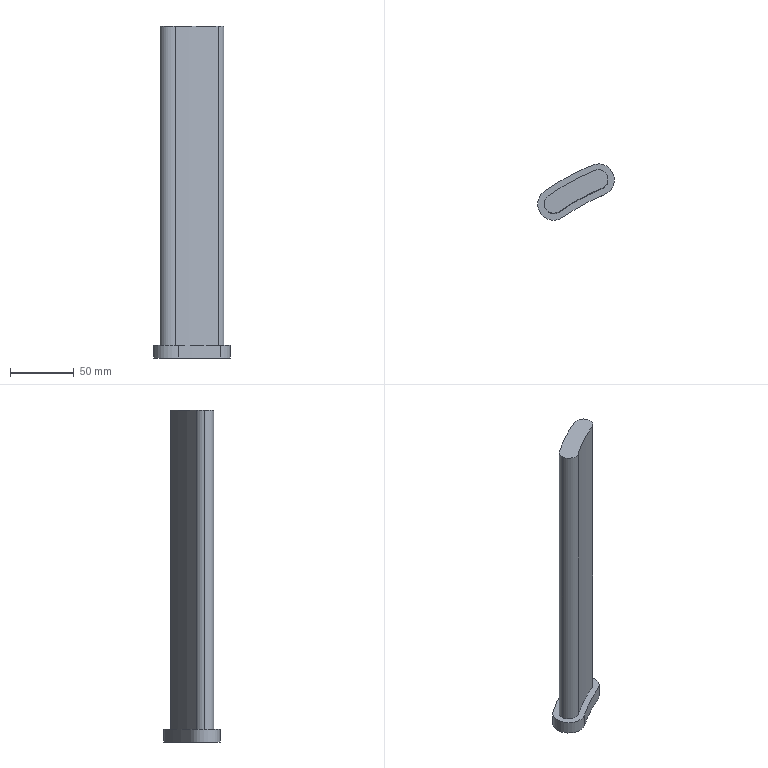Part | SolidWorks | features Extrusion 1, ICE 1 | 1 solid | 13 faces | box 60.075 x 44.074 x 260 mm | volume 209087 mm3 | cylinder 10 | plane 3 | commonest cylinder face diameters 15 x3 25 x3 355 x1 365 x1 395 x1 405 x1
STEP:
#1=CARTESIAN_POINT('',(-351.814,358.26,-240.));
#2=VERTEX_POINT('',#1);
#3=CARTESIAN_POINT('',(-359.529,346.712,-240.));
#4=VERTEX_POINT('',#3);
#5=CARTESIAN_POINT('',(-364.314,358.26,-240.));
#6=DIRECTION('',(0.,0.,-1.));
#7=DIRECTION('',(-1.,0.,0.));
#8=AXIS2_PLACEMENT_3D('',#5,#6,#7);
#9=CIRCLE('',#8,12.5);
#10=EDGE_CURVE('',#2,#4,#9,.T.);
#11=ORIENTED_EDGE('',*,*,#10,.F.);
#12=CARTESIAN_POINT('',(-351.814,358.26,-230.));
#13=VERTEX_POINT('',#12);
#14=CARTESIAN_POINT('',(-351.814,358.26,-240.));
#15=DIRECTION('',(0.,0.,1.));
#16=VECTOR('',#15,1000.);
#17=LINE('',#14,#16);
#18=EDGE_CURVE('',#2,#13,#17,.T.);
#19=ORIENTED_EDGE('',*,*,#18,.T.);
#20=CARTESIAN_POINT('',(-359.529,346.712,-230.));
#21=VERTEX_POINT('',#20);
#22=CARTESIAN_POINT('',(-364.314,358.26,-230.));
#23=DIRECTION('',(0.,0.,-1.));
#24=DIRECTION('',(-1.,0.,0.));
#25=AXIS2_PLACEMENT_3D('',#22,#23,#24);
#26=CIRCLE('',#25,12.5);
#27=EDGE_CURVE('',#13,#21,#26,.T.);
#28=ORIENTED_EDGE('',*,*,#27,.T.);
#29=CARTESIAN_POINT('',(-359.529,346.712,-240.));
#30=DIRECTION('',(0.,0.,1.));
#31=VECTOR('',#30,1000.);
#32=LINE('',#29,#31);
#33=EDGE_CURVE('',#4,#21,#32,.T.);
#34=ORIENTED_EDGE('',*,*,#33,.F.);
#35=EDGE_LOOP('',(#11,#19,#28,#34));
#36=FACE_OUTER_BOUND('',#35,.T.);
#37=CARTESIAN_POINT('',(-364.314,358.26,-240.));
#38=DIRECTION('',(0.,0.,1.));
#39=DIRECTION('',(1.,0.,0.));
#40=AXIS2_PLACEMENT_3D('',#37,#38,#39);
#41=CYLINDRICAL_SURFACE('',#40,12.5);
#42=ADVANCED_FACE('',(#36),#41,.T.);
#43=CARTESIAN_POINT('',(-406.89,339.186,20.));
#44=VERTEX_POINT('',#43);
#45=CARTESIAN_POINT('',(-395.134,333.01,20.));
#46=VERTEX_POINT('',#45);
#47=CARTESIAN_POINT('',(-399.39,339.186,20.));
#48=DIRECTION('',(0.,0.,1.));
#49=DIRECTION('',(1.,0.,0.));
#50=AXIS2_PLACEMENT_3D('',#47,#48,#49);
#51=CIRCLE('',#50,7.5);
#52=EDGE_CURVE('',#44,#46,#51,.T.);
#53=ORIENTED_EDGE('',*,*,#52,.F.);
#54=CARTESIAN_POINT('',(-406.89,339.186,-230.));
#55=VERTEX_POINT('',#54);
#56=CARTESIAN_POINT('',(-406.89,339.186,20.));
#57=DIRECTION('',(0.,0.,-1.));
#58=VECTOR('',#57,1000.);
#59=LINE('',#56,#58);
#60=EDGE_CURVE('',#44,#55,#59,.T.);
#61=ORIENTED_EDGE('',*,*,#60,.T.);
#62=CARTESIAN_POINT('',(-395.134,333.01,-230.));
#63=VERTEX_POINT('',#62);
#64=CARTESIAN_POINT('',(-399.39,339.186,-230.));
#65=DIRECTION('',(0.,0.,-1.));
#66=DIRECTION('',(1.,0.,0.));
#67=AXIS2_PLACEMENT_3D('',#64,#65,#66);
#68=CIRCLE('',#67,7.5);
#69=EDGE_CURVE('',#63,#55,#68,.T.);
#70=ORIENTED_EDGE('',*,*,#69,.F.);
#71=CARTESIAN_POINT('',(-395.134,333.01,20.));
#72=DIRECTION('',(0.,0.,-1.));
#73=VECTOR('',#72,1000.);
#74=LINE('',#71,#73);
#75=EDGE_CURVE('',#46,#63,#74,.T.);
#76=ORIENTED_EDGE('',*,*,#75,.F.);
#77=EDGE_LOOP('',(#53,#61,#70,#76));
#78=FACE_OUTER_BOUND('',#77,.T.);
#79=CARTESIAN_POINT('',(-399.39,339.186,20.));
#80=DIRECTION('',(0.,0.,-1.));
#81=DIRECTION('',(-1.,0.,0.));
#82=AXIS2_PLACEMENT_3D('',#79,#80,#81);
#83=CYLINDRICAL_SURFACE('',#82,7.5);
#84=ADVANCED_FACE('',(#78),#83,.T.);
#85=CARTESIAN_POINT('',(-361.443,351.331,20.));
#86=VERTEX_POINT('',#85);
#87=CARTESIAN_POINT('',(-361.443,351.331,-230.));
#88=VERTEX_POINT('',#87);
#89=CARTESIAN_POINT('',(-361.443,351.331,20.));
#90=DIRECTION('',(0.,0.,-1.));
#91=VECTOR('',#90,1000.);
#92=LINE('',#89,#91);
#93=EDGE_CURVE('',#86,#88,#92,.T.);
#94=ORIENTED_EDGE('',*,*,#93,.T.);
#95=CARTESIAN_POINT('',(-367.185,365.189,-230.));
#96=VERTEX_POINT('',#95);
#97=CARTESIAN_POINT('',(-364.314,358.26,-230.));
#98=DIRECTION('',(0.,0.,-1.));
#99=DIRECTION('',(1.,0.,0.));
#100=AXIS2_PLACEMENT_3D('',#97,#98,#99);
#101=CIRCLE('',#100,7.5);
#102=EDGE_CURVE('',#96,#88,#101,.T.);
#103=ORIENTED_EDGE('',*,*,#102,.F.);
#104=CARTESIAN_POINT('',(-367.185,365.189,20.));
#105=VERTEX_POINT('',#104);
#106=CARTESIAN_POINT('',(-367.185,365.189,20.));
#107=DIRECTION('',(0.,0.,-1.));
#108=VECTOR('',#107,1000.);
#109=LINE('',#106,#108);
#110=EDGE_CURVE('',#105,#96,#109,.T.);
#111=ORIENTED_EDGE('',*,*,#110,.F.);
#112=CARTESIAN_POINT('',(-364.314,358.26,20.));
#113=DIRECTION('',(0.,0.,1.));
#114=DIRECTION('',(1.,0.,0.));
#115=AXIS2_PLACEMENT_3D('',#112,#113,#114);
#116=CIRCLE('',#115,7.5);
#117=EDGE_CURVE('',#86,#105,#116,.T.);
#118=ORIENTED_EDGE('',*,*,#117,.F.);
#119=EDGE_LOOP('',(#94,#103,#111,#118));
#120=FACE_OUTER_BOUND('',#119,.T.);
#121=CARTESIAN_POINT('',(-364.314,358.26,20.));
#122=DIRECTION('',(0.,0.,-1.));
#123=DIRECTION('',(-1.,0.,0.));
#124=AXIS2_PLACEMENT_3D('',#121,#122,#123);
#125=CYLINDRICAL_SURFACE('',#124,7.5);
#126=ADVANCED_FACE('',(#120),#125,.T.);
#127=ORIENTED_EDGE('',*,*,#110,.T.);
#128=CARTESIAN_POINT('',(-403.645,345.362,-230.));
#129=VERTEX_POINT('',#128);
#130=CARTESIAN_POINT('',(-291.585,182.731,-230.));
#131=DIRECTION('',(0.,0.,-1.));
#132=DIRECTION('',(1.,0.,0.));
#133=AXIS2_PLACEMENT_3D('',#130,#131,#132);
#134=CIRCLE('',#133,197.5);
#135=EDGE_CURVE('',#129,#96,#134,.T.);
#136=ORIENTED_EDGE('',*,*,#135,.F.);
#137=CARTESIAN_POINT('',(-403.645,345.362,20.));
#138=VERTEX_POINT('',#137);
#139=CARTESIAN_POINT('',(-403.645,345.362,20.));
#140=DIRECTION('',(0.,0.,-1.));
#141=VECTOR('',#140,1000.);
#142=LINE('',#139,#141);
#143=EDGE_CURVE('',#138,#129,#142,.T.);
#144=ORIENTED_EDGE('',*,*,#143,.F.);
#145=CARTESIAN_POINT('',(-291.585,182.731,20.));
#146=DIRECTION('',(0.,0.,1.));
#147=DIRECTION('',(1.,0.,0.));
#148=AXIS2_PLACEMENT_3D('',#145,#146,#147);
#149=CIRCLE('',#148,197.5);
#150=EDGE_CURVE('',#105,#138,#149,.T.);
#151=ORIENTED_EDGE('',*,*,#150,.F.);
#152=EDGE_LOOP('',(#127,#136,#144,#151));
#153=FACE_OUTER_BOUND('',#152,.T.);
#154=CARTESIAN_POINT('',(-291.585,182.731,20.));
#155=DIRECTION('',(0.,0.,-1.));
#156=DIRECTION('',(-1.,0.,0.));
#157=AXIS2_PLACEMENT_3D('',#154,#155,#156);
#158=CYLINDRICAL_SURFACE('',#157,197.5);
#159=ADVANCED_FACE('',(#153),#158,.T.);
#160=ORIENTED_EDGE('',*,*,#60,.F.);
#161=CARTESIAN_POINT('',(-399.39,339.186,20.));
#162=DIRECTION('',(0.,0.,1.));
#163=DIRECTION('',(1.,0.,0.));
#164=AXIS2_PLACEMENT_3D('',#161,#162,#163);
#165=CIRCLE('',#164,7.5);
#166=EDGE_CURVE('',#138,#44,#165,.T.);
#167=ORIENTED_EDGE('',*,*,#166,.F.);
#168=ORIENTED_EDGE('',*,*,#143,.T.);
#169=CARTESIAN_POINT('',(-399.39,339.186,-230.));
#170=DIRECTION('',(0.,0.,-1.));
#171=DIRECTION('',(1.,0.,0.));
#172=AXIS2_PLACEMENT_3D('',#169,#170,#171);
#173=CIRCLE('',#172,7.5);
#174=EDGE_CURVE('',#55,#129,#173,.T.);
#175=ORIENTED_EDGE('',*,*,#174,.F.);
#176=EDGE_LOOP('',(#160,#167,#168,#175));
#177=FACE_OUTER_BOUND('',#176,.T.);
#178=CARTESIAN_POINT('',(-399.39,339.186,20.));
#179=DIRECTION('',(0.,0.,-1.));
#180=DIRECTION('',(-1.,0.,0.));
#181=AXIS2_PLACEMENT_3D('',#178,#179,#180);
#182=CYLINDRICAL_SURFACE('',#181,7.5);
#183=ADVANCED_FACE('',(#177),#182,.T.);
#184=ORIENTED_EDGE('',*,*,#75,.T.);
#185=CARTESIAN_POINT('',(-291.585,182.731,-230.));
#186=DIRECTION('',(0.,0.,1.));
#187=DIRECTION('',(1.,0.,0.));
#188=AXIS2_PLACEMENT_3D('',#185,#186,#187);
#189=CIRCLE('',#188,182.5);
#190=EDGE_CURVE('',#88,#63,#189,.T.);
#191=ORIENTED_EDGE('',*,*,#190,.F.);
#192=ORIENTED_EDGE('',*,*,#93,.F.);
#193=CARTESIAN_POINT('',(-291.585,182.731,20.));
#194=DIRECTION('',(0.,0.,-1.));
#195=DIRECTION('',(1.,0.,0.));
#196=AXIS2_PLACEMENT_3D('',#193,#194,#195);
#197=CIRCLE('',#196,182.5);
#198=EDGE_CURVE('',#46,#86,#197,.T.);
#199=ORIENTED_EDGE('',*,*,#198,.F.);
#200=EDGE_LOOP('',(#184,#191,#192,#199));
#201=FACE_OUTER_BOUND('',#200,.T.);
#202=CARTESIAN_POINT('',(-291.585,182.731,20.));
#203=DIRECTION('',(0.,0.,-1.));
#204=DIRECTION('',(-1.,0.,0.));
#205=AXIS2_PLACEMENT_3D('',#202,#203,#204);
#206=CYLINDRICAL_SURFACE('',#205,182.5);
#207=ADVANCED_FACE('',(#201),#206,.F.);
#208=ORIENTED_EDGE('',*,*,#117,.T.);
#209=ORIENTED_EDGE('',*,*,#150,.T.);
#210=ORIENTED_EDGE('',*,*,#166,.T.);
#211=ORIENTED_EDGE('',*,*,#52,.T.);
#212=ORIENTED_EDGE('',*,*,#198,.T.);
#213=EDGE_LOOP('',(#208,#209,#210,#211,#212));
#214=FACE_OUTER_BOUND('',#213,.T.);
#215=CARTESIAN_POINT('',(-327.95,270.495,20.));
#216=DIRECTION('',(0.,0.,1.));
#217=DIRECTION('',(1.,0.,0.));
#218=AXIS2_PLACEMENT_3D('',#215,#216,#217);
#219=PLANE('',#218);
#220=ADVANCED_FACE('',(#214),#219,.T.);
#221=CARTESIAN_POINT('',(-392.297,328.893,-230.));
#222=VERTEX_POINT('',#221);
#223=CARTESIAN_POINT('',(-406.482,349.479,-230.));
#224=VERTEX_POINT('',#223);
#225=CARTESIAN_POINT('',(-399.39,339.186,-230.));
#226=DIRECTION('',(0.,0.,-1.));
#227=DIRECTION('',(-1.,0.,0.));
#228=AXIS2_PLACEMENT_3D('',#225,#226,#227);
#229=CIRCLE('',#228,12.5);
#230=EDGE_CURVE('',#222,#224,#229,.T.);
#231=ORIENTED_EDGE('',*,*,#230,.T.);
#232=CARTESIAN_POINT('',(-406.482,349.479,-240.));
#233=VERTEX_POINT('',#232);
#234=CARTESIAN_POINT('',(-406.482,349.479,-240.));
#235=DIRECTION('',(0.,0.,1.));
#236=VECTOR('',#235,1000.);
#237=LINE('',#234,#236);
#238=EDGE_CURVE('',#233,#224,#237,.T.);
#239=ORIENTED_EDGE('',*,*,#238,.F.);
#240=CARTESIAN_POINT('',(-392.297,328.893,-240.));
#241=VERTEX_POINT('',#240);
#242=CARTESIAN_POINT('',(-399.39,339.186,-240.));
#243=DIRECTION('',(0.,0.,-1.));
#244=DIRECTION('',(-1.,0.,0.));
#245=AXIS2_PLACEMENT_3D('',#242,#243,#244);
#246=CIRCLE('',#245,12.5);
#247=EDGE_CURVE('',#241,#233,#246,.T.);
#248=ORIENTED_EDGE('',*,*,#247,.F.);
#249=CARTESIAN_POINT('',(-392.297,328.893,-240.));
#250=DIRECTION('',(0.,0.,1.));
#251=VECTOR('',#250,1000.);
#252=LINE('',#249,#251);
#253=EDGE_CURVE('',#241,#222,#252,.T.);
#254=ORIENTED_EDGE('',*,*,#253,.T.);
#255=EDGE_LOOP('',(#231,#239,#248,#254));
#256=FACE_OUTER_BOUND('',#255,.T.);
#257=CARTESIAN_POINT('',(-399.39,339.186,-240.));
#258=DIRECTION('',(0.,0.,1.));
#259=DIRECTION('',(1.,0.,0.));
#260=AXIS2_PLACEMENT_3D('',#257,#258,#259);
#261=CYLINDRICAL_SURFACE('',#260,12.5);
#262=ADVANCED_FACE('',(#256),#261,.T.);
#263=CARTESIAN_POINT('',(-369.099,369.808,-230.));
#264=VERTEX_POINT('',#263);
#265=CARTESIAN_POINT('',(-291.585,182.731,-230.));
#266=DIRECTION('',(0.,0.,-1.));
#267=DIRECTION('',(-1.,0.,0.));
#268=AXIS2_PLACEMENT_3D('',#265,#266,#267);
#269=CIRCLE('',#268,202.5);
#270=EDGE_CURVE('',#224,#264,#269,.T.);
#271=ORIENTED_EDGE('',*,*,#270,.T.);
#272=CARTESIAN_POINT('',(-369.099,369.808,-240.));
#273=VERTEX_POINT('',#272);
#274=CARTESIAN_POINT('',(-369.099,369.808,-240.));
#275=DIRECTION('',(0.,0.,1.));
#276=VECTOR('',#275,1000.);
#277=LINE('',#274,#276);
#278=EDGE_CURVE('',#273,#264,#277,.T.);
#279=ORIENTED_EDGE('',*,*,#278,.F.);
#280=CARTESIAN_POINT('',(-291.585,182.731,-240.));
#281=DIRECTION('',(0.,0.,-1.));
#282=DIRECTION('',(-1.,0.,0.));
#283=AXIS2_PLACEMENT_3D('',#280,#281,#282);
#284=CIRCLE('',#283,202.5);
#285=EDGE_CURVE('',#233,#273,#284,.T.);
#286=ORIENTED_EDGE('',*,*,#285,.F.);
#287=ORIENTED_EDGE('',*,*,#238,.T.);
#288=EDGE_LOOP('',(#271,#279,#286,#287));
#289=FACE_OUTER_BOUND('',#288,.T.);
#290=CARTESIAN_POINT('',(-291.585,182.731,-240.));
#291=DIRECTION('',(0.,0.,1.));
#292=DIRECTION('',(1.,0.,0.));
#293=AXIS2_PLACEMENT_3D('',#290,#291,#292);
#294=CYLINDRICAL_SURFACE('',#293,202.5);
#295=ADVANCED_FACE('',(#289),#294,.T.);
#296=ORIENTED_EDGE('',*,*,#18,.F.);
#297=CARTESIAN_POINT('',(-364.314,358.26,-240.));
#298=DIRECTION('',(0.,0.,-1.));
#299=DIRECTION('',(-1.,0.,0.));
#300=AXIS2_PLACEMENT_3D('',#297,#298,#299);
#301=CIRCLE('',#300,12.5);
#302=EDGE_CURVE('',#273,#2,#301,.T.);
#303=ORIENTED_EDGE('',*,*,#302,.F.);
#304=ORIENTED_EDGE('',*,*,#278,.T.);
#305=CARTESIAN_POINT('',(-364.314,358.26,-230.));
#306=DIRECTION('',(0.,0.,-1.));
#307=DIRECTION('',(-1.,0.,0.));
#308=AXIS2_PLACEMENT_3D('',#305,#306,#307);
#309=CIRCLE('',#308,12.5);
#310=EDGE_CURVE('',#264,#13,#309,.T.);
#311=ORIENTED_EDGE('',*,*,#310,.T.);
#312=EDGE_LOOP('',(#296,#303,#304,#311));
#313=FACE_OUTER_BOUND('',#312,.T.);
#314=CARTESIAN_POINT('',(-364.314,358.26,-240.));
#315=DIRECTION('',(0.,0.,1.));
#316=DIRECTION('',(1.,0.,0.));
#317=AXIS2_PLACEMENT_3D('',#314,#315,#316);
#318=CYLINDRICAL_SURFACE('',#317,12.5);
#319=ADVANCED_FACE('',(#313),#318,.T.);
#320=CARTESIAN_POINT('',(-291.585,182.731,-230.));
#321=DIRECTION('',(0.,0.,1.));
#322=DIRECTION('',(-1.,0.,0.));
#323=AXIS2_PLACEMENT_3D('',#320,#321,#322);
#324=CIRCLE('',#323,177.5);
#325=EDGE_CURVE('',#21,#222,#324,.T.);
#326=ORIENTED_EDGE('',*,*,#325,.T.);
#327=ORIENTED_EDGE('',*,*,#253,.F.);
#328=CARTESIAN_POINT('',(-291.585,182.731,-240.));
#329=DIRECTION('',(0.,0.,1.));
#330=DIRECTION('',(-1.,0.,0.));
#331=AXIS2_PLACEMENT_3D('',#328,#329,#330);
#332=CIRCLE('',#331,177.5);
#333=EDGE_CURVE('',#4,#241,#332,.T.);
#334=ORIENTED_EDGE('',*,*,#333,.F.);
#335=ORIENTED_EDGE('',*,*,#33,.T.);
#336=EDGE_LOOP('',(#326,#327,#334,#335));
#337=FACE_OUTER_BOUND('',#336,.T.);
#338=CARTESIAN_POINT('',(-291.585,182.731,-240.));
#339=DIRECTION('',(0.,0.,1.));
#340=DIRECTION('',(1.,0.,0.));
#341=AXIS2_PLACEMENT_3D('',#338,#339,#340);
#342=CYLINDRICAL_SURFACE('',#341,177.5);
#343=ADVANCED_FACE('',(#337),#342,.F.);
#344=ORIENTED_EDGE('',*,*,#247,.T.);
#345=ORIENTED_EDGE('',*,*,#285,.T.);
#346=ORIENTED_EDGE('',*,*,#302,.T.);
#347=ORIENTED_EDGE('',*,*,#10,.T.);
#348=ORIENTED_EDGE('',*,*,#333,.T.);
#349=EDGE_LOOP('',(#344,#345,#346,#347,#348));
#350=FACE_OUTER_BOUND('',#349,.T.);
#351=CARTESIAN_POINT('',(-345.487,260.958,-240.));
#352=DIRECTION('',(0.,0.,-1.));
#353=DIRECTION('',(-1.,0.,0.));
#354=AXIS2_PLACEMENT_3D('',#351,#352,#353);
#355=PLANE('',#354);
#356=ADVANCED_FACE('',(#350),#355,.T.);
#357=ORIENTED_EDGE('',*,*,#135,.T.);
#358=ORIENTED_EDGE('',*,*,#102,.T.);
#359=ORIENTED_EDGE('',*,*,#190,.T.);
#360=ORIENTED_EDGE('',*,*,#69,.T.);
#361=ORIENTED_EDGE('',*,*,#174,.T.);
#362=EDGE_LOOP('',(#357,#358,#359,#360,#361));
#363=FACE_BOUND('',#362,.T.);
#364=ORIENTED_EDGE('',*,*,#230,.F.);
#365=ORIENTED_EDGE('',*,*,#325,.F.);
#366=ORIENTED_EDGE('',*,*,#27,.F.);
#367=ORIENTED_EDGE('',*,*,#310,.F.);
#368=ORIENTED_EDGE('',*,*,#270,.F.);
#369=EDGE_LOOP('',(#364,#365,#366,#367,#368));
#370=FACE_OUTER_BOUND('',#369,.T.);
#371=CARTESIAN_POINT('',(-345.487,260.958,-230.));
#372=DIRECTION('',(0.,0.,-1.));
#373=DIRECTION('',(-1.,0.,0.));
#374=AXIS2_PLACEMENT_3D('',#371,#372,#373);
#375=PLANE('',#374);
#376=ADVANCED_FACE('',(#363,#370),#375,.F.);
#377=CLOSED_SHELL('',(#42,#84,#126,#159,#183,#207,#220,#262,#295,#319,#343,#356,#376));
#378=MANIFOLD_SOLID_BREP('',#377);
#379=CARTESIAN_POINT('',(0.,0.,0.));
#380=DIRECTION('',(0.,0.,1.));
#381=DIRECTION('',(1.,0.,0.));
#382=AXIS2_PLACEMENT_3D('',#379,#380,#381);
#383=(LENGTH_UNIT()NAMED_UNIT(*)SI_UNIT(.MILLI.,.METRE.));
#384=UNCERTAINTY_MEASURE_WITH_UNIT(LENGTH_MEASURE(0.00001),#383,'','');
#385=(NAMED_UNIT(*)PLANE_ANGLE_UNIT()SI_UNIT($,.RADIAN.));
#386=(NAMED_UNIT(*)SI_UNIT($,.STERADIAN.)SOLID_ANGLE_UNIT());
#387=(GEOMETRIC_REPRESENTATION_CONTEXT(3)GLOBAL_UNCERTAINTY_ASSIGNED_CONTEXT((#384))GLOBAL_UNIT_ASSIGNED_CONTEXT((#383,#385,#386))REPRESENTATION_CONTEXT('',''));
#388=ADVANCED_BREP_SHAPE_REPRESENTATION('',(#378,#382),#387);